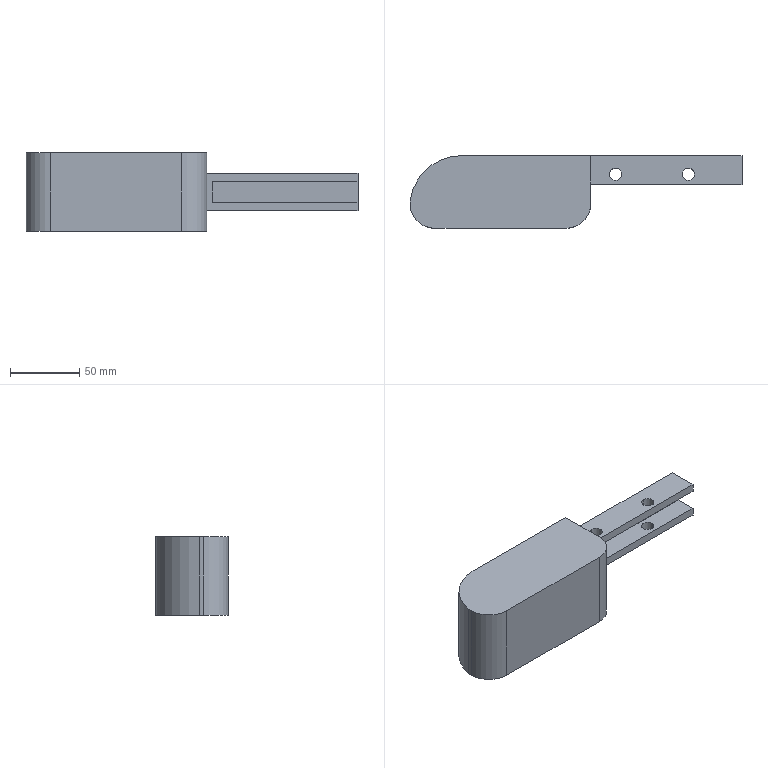Part | SolidWorks | features BaseBody 1, ICE 1 | 1 solid | 25 faces | box 239.768 x 52.5 x 57 mm | volume 402739 mm3 | plane 13 | cylinder 12 | commonest cylinder face diameters 9 x8 36 x3 75 x1
STEP:
#1=CARTESIAN_POINT('',(0.2322,-13.5,42.));
#2=VERTEX_POINT('',#1);
#3=CARTESIAN_POINT('',(18.232,-31.5,42.));
#4=VERTEX_POINT('',#3);
#5=CARTESIAN_POINT('',(18.232,-13.5,42.));
#6=DIRECTION('',(0.,0.,1.));
#7=DIRECTION('',(-1.,0.,0.));
#8=AXIS2_PLACEMENT_3D('',#5,#6,#7);
#9=CIRCLE('',#8,18.);
#10=EDGE_CURVE('',#2,#4,#9,.T.);
#11=ORIENTED_EDGE('',*,*,#10,.F.);
#12=CARTESIAN_POINT('',(0.2322,-13.5,-15.));
#13=VERTEX_POINT('',#12);
#14=CARTESIAN_POINT('',(0.2322,-13.5,42.));
#15=DIRECTION('',(0.,0.,-1.));
#16=VECTOR('',#15,1000.);
#17=LINE('',#14,#16);
#18=EDGE_CURVE('',#2,#13,#17,.T.);
#19=ORIENTED_EDGE('',*,*,#18,.T.);
#20=CARTESIAN_POINT('',(18.232,-31.5,-15.));
#21=VERTEX_POINT('',#20);
#22=CARTESIAN_POINT('',(18.232,-13.5,-15.));
#23=DIRECTION('',(0.,0.,-1.));
#24=DIRECTION('',(-1.,0.,0.));
#25=AXIS2_PLACEMENT_3D('',#22,#23,#24);
#26=CIRCLE('',#25,18.);
#27=EDGE_CURVE('',#21,#13,#26,.T.);
#28=ORIENTED_EDGE('',*,*,#27,.F.);
#29=CARTESIAN_POINT('',(18.232,-31.5,13.5));
#30=DIRECTION('',(0.,0.,-1.));
#31=VECTOR('',#30,1000.);
#32=LINE('',#29,#31);
#33=EDGE_CURVE('',#4,#21,#32,.T.);
#34=ORIENTED_EDGE('',*,*,#33,.F.);
#35=EDGE_LOOP('',(#11,#19,#28,#34));
#36=FACE_OUTER_BOUND('',#35,.T.);
#37=CARTESIAN_POINT('',(18.232,-13.5,42.));
#38=DIRECTION('',(0.,0.,-1.));
#39=DIRECTION('',(-1.,0.,0.));
#40=AXIS2_PLACEMENT_3D('',#37,#38,#39);
#41=CYLINDRICAL_SURFACE('',#40,18.);
#42=ADVANCED_FACE('',(#36),#41,.T.);
#43=CARTESIAN_POINT('',(144.21,7.5,6.));
#44=VERTEX_POINT('',#43);
#45=CARTESIAN_POINT('',(153.21,7.5,6.));
#46=VERTEX_POINT('',#45);
#47=CARTESIAN_POINT('',(148.71,7.5,6.));
#48=DIRECTION('',(0.,0.,1.));
#49=DIRECTION('',(-1.,0.,0.));
#50=AXIS2_PLACEMENT_3D('',#47,#48,#49);
#51=CIRCLE('',#50,4.5);
#52=EDGE_CURVE('',#44,#46,#51,.T.);
#53=ORIENTED_EDGE('',*,*,#52,.T.);
#54=CARTESIAN_POINT('',(153.21,7.5,0.));
#55=VERTEX_POINT('',#54);
#56=CARTESIAN_POINT('',(153.21,7.5,6.));
#57=DIRECTION('',(0.,0.,-1.));
#58=VECTOR('',#57,1000.);
#59=LINE('',#56,#58);
#60=EDGE_CURVE('',#46,#55,#59,.T.);
#61=ORIENTED_EDGE('',*,*,#60,.T.);
#62=CARTESIAN_POINT('',(144.21,7.5,0.));
#63=VERTEX_POINT('',#62);
#64=CARTESIAN_POINT('',(148.71,7.5,0.));
#65=DIRECTION('',(0.,0.,1.));
#66=DIRECTION('',(-1.,0.,0.));
#67=AXIS2_PLACEMENT_3D('',#64,#65,#66);
#68=CIRCLE('',#67,4.5);
#69=EDGE_CURVE('',#63,#55,#68,.T.);
#70=ORIENTED_EDGE('',*,*,#69,.F.);
#71=CARTESIAN_POINT('',(144.21,7.5,6.));
#72=DIRECTION('',(0.,0.,-1.));
#73=VECTOR('',#72,1000.);
#74=LINE('',#71,#73);
#75=EDGE_CURVE('',#44,#63,#74,.T.);
#76=ORIENTED_EDGE('',*,*,#75,.F.);
#77=EDGE_LOOP('',(#53,#61,#70,#76));
#78=FACE_OUTER_BOUND('',#77,.T.);
#79=CARTESIAN_POINT('',(148.71,7.5,6.));
#80=DIRECTION('',(0.,0.,-1.));
#81=DIRECTION('',(-1.,0.,0.));
#82=AXIS2_PLACEMENT_3D('',#79,#80,#81);
#83=CYLINDRICAL_SURFACE('',#82,4.5);
#84=ADVANCED_FACE('',(#78),#83,.F.);
#85=CARTESIAN_POINT('',(196.71,7.5,6.));
#86=VERTEX_POINT('',#85);
#87=CARTESIAN_POINT('',(205.71,7.5,6.));
#88=VERTEX_POINT('',#87);
#89=CARTESIAN_POINT('',(201.21,7.5,6.));
#90=DIRECTION('',(0.,0.,1.));
#91=DIRECTION('',(-1.,0.,0.));
#92=AXIS2_PLACEMENT_3D('',#89,#90,#91);
#93=CIRCLE('',#92,4.5);
#94=EDGE_CURVE('',#86,#88,#93,.T.);
#95=ORIENTED_EDGE('',*,*,#94,.T.);
#96=CARTESIAN_POINT('',(205.71,7.5,0.));
#97=VERTEX_POINT('',#96);
#98=CARTESIAN_POINT('',(205.71,7.5,6.));
#99=DIRECTION('',(0.,0.,-1.));
#100=VECTOR('',#99,1000.);
#101=LINE('',#98,#100);
#102=EDGE_CURVE('',#88,#97,#101,.T.);
#103=ORIENTED_EDGE('',*,*,#102,.T.);
#104=CARTESIAN_POINT('',(196.71,7.5,0.));
#105=VERTEX_POINT('',#104);
#106=CARTESIAN_POINT('',(201.21,7.5,0.));
#107=DIRECTION('',(0.,0.,1.));
#108=DIRECTION('',(-1.,0.,0.));
#109=AXIS2_PLACEMENT_3D('',#106,#107,#108);
#110=CIRCLE('',#109,4.5);
#111=EDGE_CURVE('',#105,#97,#110,.T.);
#112=ORIENTED_EDGE('',*,*,#111,.F.);
#113=CARTESIAN_POINT('',(196.71,7.5,6.));
#114=DIRECTION('',(0.,0.,-1.));
#115=VECTOR('',#114,1000.);
#116=LINE('',#113,#115);
#117=EDGE_CURVE('',#86,#105,#116,.T.);
#118=ORIENTED_EDGE('',*,*,#117,.F.);
#119=EDGE_LOOP('',(#95,#103,#112,#118));
#120=FACE_OUTER_BOUND('',#119,.T.);
#121=CARTESIAN_POINT('',(201.21,7.5,6.));
#122=DIRECTION('',(0.,0.,-1.));
#123=DIRECTION('',(-1.,0.,0.));
#124=AXIS2_PLACEMENT_3D('',#121,#122,#123);
#125=CYLINDRICAL_SURFACE('',#124,4.5);
#126=ADVANCED_FACE('',(#120),#125,.F.);
#127=CARTESIAN_POINT('',(148.71,12.,27.));
#128=VERTEX_POINT('',#127);
#129=CARTESIAN_POINT('',(148.71,3.,27.));
#130=VERTEX_POINT('',#129);
#131=CARTESIAN_POINT('',(148.71,7.5,27.));
#132=DIRECTION('',(0.,0.,1.));
#133=DIRECTION('',(0.,1.,0.));
#134=AXIS2_PLACEMENT_3D('',#131,#132,#133);
#135=CIRCLE('',#134,4.5);
#136=EDGE_CURVE('',#128,#130,#135,.T.);
#137=ORIENTED_EDGE('',*,*,#136,.T.);
#138=CARTESIAN_POINT('',(148.71,3.,21.));
#139=VERTEX_POINT('',#138);
#140=CARTESIAN_POINT('',(148.71,3.,27.));
#141=DIRECTION('',(0.,0.,-1.));
#142=VECTOR('',#141,1000.);
#143=LINE('',#140,#142);
#144=EDGE_CURVE('',#130,#139,#143,.T.);
#145=ORIENTED_EDGE('',*,*,#144,.T.);
#146=CARTESIAN_POINT('',(148.71,12.,21.));
#147=VERTEX_POINT('',#146);
#148=CARTESIAN_POINT('',(148.71,7.5,21.));
#149=DIRECTION('',(0.,0.,-1.));
#150=DIRECTION('',(0.,1.,0.));
#151=AXIS2_PLACEMENT_3D('',#148,#149,#150);
#152=CIRCLE('',#151,4.5);
#153=EDGE_CURVE('',#139,#147,#152,.T.);
#154=ORIENTED_EDGE('',*,*,#153,.T.);
#155=CARTESIAN_POINT('',(148.71,12.,27.));
#156=DIRECTION('',(0.,0.,-1.));
#157=VECTOR('',#156,1000.);
#158=LINE('',#155,#157);
#159=EDGE_CURVE('',#128,#147,#158,.T.);
#160=ORIENTED_EDGE('',*,*,#159,.F.);
#161=EDGE_LOOP('',(#137,#145,#154,#160));
#162=FACE_OUTER_BOUND('',#161,.T.);
#163=CARTESIAN_POINT('',(148.71,7.5,27.));
#164=DIRECTION('',(0.,0.,-1.));
#165=DIRECTION('',(0.,1.,0.));
#166=AXIS2_PLACEMENT_3D('',#163,#164,#165);
#167=CYLINDRICAL_SURFACE('',#166,4.5);
#168=ADVANCED_FACE('',(#162),#167,.F.);
#169=CARTESIAN_POINT('',(201.21,12.,27.));
#170=VERTEX_POINT('',#169);
#171=CARTESIAN_POINT('',(201.21,3.,27.));
#172=VERTEX_POINT('',#171);
#173=CARTESIAN_POINT('',(201.21,7.5,27.));
#174=DIRECTION('',(0.,0.,1.));
#175=DIRECTION('',(0.,1.,0.));
#176=AXIS2_PLACEMENT_3D('',#173,#174,#175);
#177=CIRCLE('',#176,4.5);
#178=EDGE_CURVE('',#170,#172,#177,.T.);
#179=ORIENTED_EDGE('',*,*,#178,.T.);
#180=CARTESIAN_POINT('',(201.21,3.,21.));
#181=VERTEX_POINT('',#180);
#182=CARTESIAN_POINT('',(201.21,3.,27.));
#183=DIRECTION('',(0.,0.,-1.));
#184=VECTOR('',#183,1000.);
#185=LINE('',#182,#184);
#186=EDGE_CURVE('',#172,#181,#185,.T.);
#187=ORIENTED_EDGE('',*,*,#186,.T.);
#188=CARTESIAN_POINT('',(201.21,12.,21.));
#189=VERTEX_POINT('',#188);
#190=CARTESIAN_POINT('',(201.21,7.5,21.));
#191=DIRECTION('',(0.,0.,-1.));
#192=DIRECTION('',(0.,1.,0.));
#193=AXIS2_PLACEMENT_3D('',#190,#191,#192);
#194=CIRCLE('',#193,4.5);
#195=EDGE_CURVE('',#181,#189,#194,.T.);
#196=ORIENTED_EDGE('',*,*,#195,.T.);
#197=CARTESIAN_POINT('',(201.21,12.,27.));
#198=DIRECTION('',(0.,0.,-1.));
#199=VECTOR('',#198,1000.);
#200=LINE('',#197,#199);
#201=EDGE_CURVE('',#170,#189,#200,.T.);
#202=ORIENTED_EDGE('',*,*,#201,.F.);
#203=EDGE_LOOP('',(#179,#187,#196,#202));
#204=FACE_OUTER_BOUND('',#203,.T.);
#205=CARTESIAN_POINT('',(201.21,7.5,27.));
#206=DIRECTION('',(0.,0.,-1.));
#207=DIRECTION('',(0.,1.,0.));
#208=AXIS2_PLACEMENT_3D('',#205,#206,#207);
#209=CYLINDRICAL_SURFACE('',#208,4.5);
#210=ADVANCED_FACE('',(#204),#209,.F.);
#211=ORIENTED_EDGE('',*,*,#18,.F.);
#212=CARTESIAN_POINT('',(0.4464,-10.731,42.));
#213=VERTEX_POINT('',#212);
#214=CARTESIAN_POINT('',(18.232,-13.5,42.));
#215=DIRECTION('',(0.,0.,1.));
#216=DIRECTION('',(-1.,0.,0.));
#217=AXIS2_PLACEMENT_3D('',#214,#215,#216);
#218=CIRCLE('',#217,18.);
#219=EDGE_CURVE('',#213,#2,#218,.T.);
#220=ORIENTED_EDGE('',*,*,#219,.F.);
#221=CARTESIAN_POINT('',(0.4464,-10.731,-15.));
#222=VERTEX_POINT('',#221);
#223=CARTESIAN_POINT('',(0.4464,-10.731,13.5));
#224=DIRECTION('',(0.,0.,1.));
#225=VECTOR('',#224,1000.);
#226=LINE('',#223,#225);
#227=EDGE_CURVE('',#222,#213,#226,.T.);
#228=ORIENTED_EDGE('',*,*,#227,.F.);
#229=CARTESIAN_POINT('',(18.232,-13.5,-15.));
#230=DIRECTION('',(0.,0.,-1.));
#231=DIRECTION('',(-1.,0.,0.));
#232=AXIS2_PLACEMENT_3D('',#229,#230,#231);
#233=CIRCLE('',#232,18.);
#234=EDGE_CURVE('',#13,#222,#233,.T.);
#235=ORIENTED_EDGE('',*,*,#234,.F.);
#236=EDGE_LOOP('',(#211,#220,#228,#235));
#237=FACE_OUTER_BOUND('',#236,.T.);
#238=CARTESIAN_POINT('',(18.232,-13.5,42.));
#239=DIRECTION('',(0.,0.,-1.));
#240=DIRECTION('',(-1.,0.,0.));
#241=AXIS2_PLACEMENT_3D('',#238,#239,#240);
#242=CYLINDRICAL_SURFACE('',#241,18.);
#243=ADVANCED_FACE('',(#237),#242,.T.);
#244=CARTESIAN_POINT('',(130.767,21.,42.));
#245=VERTEX_POINT('',#244);
#246=CARTESIAN_POINT('',(130.767,-13.5,42.));
#247=VERTEX_POINT('',#246);
#248=CARTESIAN_POINT('',(130.767,-5.25,42.));
#249=DIRECTION('',(0.,-1.,0.));
#250=VECTOR('',#249,1000.);
#251=LINE('',#248,#250);
#252=EDGE_CURVE('',#245,#247,#251,.T.);
#253=ORIENTED_EDGE('',*,*,#252,.F.);
#254=CARTESIAN_POINT('',(37.5,21.,42.));
#255=VERTEX_POINT('',#254);
#256=CARTESIAN_POINT('',(65.108,21.,42.));
#257=DIRECTION('',(1.,0.,0.));
#258=VECTOR('',#257,1000.);
#259=LINE('',#256,#258);
#260=EDGE_CURVE('',#255,#245,#259,.T.);
#261=ORIENTED_EDGE('',*,*,#260,.F.);
#262=CARTESIAN_POINT('',(37.5,-16.5,42.));
#263=DIRECTION('',(0.,0.,-1.));
#264=DIRECTION('',(-1.,0.,0.));
#265=AXIS2_PLACEMENT_3D('',#262,#263,#264);
#266=CIRCLE('',#265,37.5);
#267=EDGE_CURVE('',#213,#255,#266,.T.);
#268=ORIENTED_EDGE('',*,*,#267,.F.);
#269=ORIENTED_EDGE('',*,*,#219,.T.);
#270=ORIENTED_EDGE('',*,*,#10,.T.);
#271=CARTESIAN_POINT('',(112.767,-31.5,42.));
#272=VERTEX_POINT('',#271);
#273=CARTESIAN_POINT('',(65.108,-31.5,42.));
#274=DIRECTION('',(-1.,0.,0.));
#275=VECTOR('',#274,1000.);
#276=LINE('',#273,#275);
#277=EDGE_CURVE('',#272,#4,#276,.T.);
#278=ORIENTED_EDGE('',*,*,#277,.F.);
#279=CARTESIAN_POINT('',(112.767,-13.5,42.));
#280=DIRECTION('',(0.,0.,-1.));
#281=DIRECTION('',(-1.,0.,0.));
#282=AXIS2_PLACEMENT_3D('',#279,#280,#281);
#283=CIRCLE('',#282,18.);
#284=EDGE_CURVE('',#247,#272,#283,.T.);
#285=ORIENTED_EDGE('',*,*,#284,.F.);
#286=EDGE_LOOP('',(#253,#261,#268,#269,#270,#278,#285));
#287=FACE_OUTER_BOUND('',#286,.T.);
#288=CARTESIAN_POINT('',(130.767,-31.5,42.));
#289=DIRECTION('',(0.,0.,-1.));
#290=DIRECTION('',(-1.,0.,0.));
#291=AXIS2_PLACEMENT_3D('',#288,#289,#290);
#292=PLANE('',#291);
#293=ADVANCED_FACE('',(#287),#292,.F.);
#294=CARTESIAN_POINT('',(112.767,-31.5,-15.));
#295=VERTEX_POINT('',#294);
#296=CARTESIAN_POINT('',(65.108,-31.5,-15.));
#297=DIRECTION('',(1.,0.,0.));
#298=VECTOR('',#297,1000.);
#299=LINE('',#296,#298);
#300=EDGE_CURVE('',#21,#295,#299,.T.);
#301=ORIENTED_EDGE('',*,*,#300,.F.);
#302=ORIENTED_EDGE('',*,*,#27,.T.);
#303=ORIENTED_EDGE('',*,*,#234,.T.);
#304=CARTESIAN_POINT('',(37.5,21.,-15.));
#305=VERTEX_POINT('',#304);
#306=CARTESIAN_POINT('',(37.5,-16.5,-15.));
#307=DIRECTION('',(0.,0.,1.));
#308=DIRECTION('',(-1.,0.,0.));
#309=AXIS2_PLACEMENT_3D('',#306,#307,#308);
#310=CIRCLE('',#309,37.5);
#311=EDGE_CURVE('',#305,#222,#310,.T.);
#312=ORIENTED_EDGE('',*,*,#311,.F.);
#313=CARTESIAN_POINT('',(130.767,21.,-15.));
#314=VERTEX_POINT('',#313);
#315=CARTESIAN_POINT('',(65.108,21.,-15.));
#316=DIRECTION('',(-1.,0.,0.));
#317=VECTOR('',#316,1000.);
#318=LINE('',#315,#317);
#319=EDGE_CURVE('',#314,#305,#318,.T.);
#320=ORIENTED_EDGE('',*,*,#319,.F.);
#321=CARTESIAN_POINT('',(130.767,-13.5,-15.));
#322=VERTEX_POINT('',#321);
#323=CARTESIAN_POINT('',(130.767,-5.25,-15.));
#324=DIRECTION('',(0.,1.,0.));
#325=VECTOR('',#324,1000.);
#326=LINE('',#323,#325);
#327=EDGE_CURVE('',#322,#314,#326,.T.);
#328=ORIENTED_EDGE('',*,*,#327,.F.);
#329=CARTESIAN_POINT('',(112.767,-13.5,-15.));
#330=DIRECTION('',(0.,0.,1.));
#331=DIRECTION('',(-1.,0.,0.));
#332=AXIS2_PLACEMENT_3D('',#329,#330,#331);
#333=CIRCLE('',#332,18.);
#334=EDGE_CURVE('',#295,#322,#333,.T.);
#335=ORIENTED_EDGE('',*,*,#334,.F.);
#336=EDGE_LOOP('',(#301,#302,#303,#312,#320,#328,#335));
#337=FACE_OUTER_BOUND('',#336,.T.);
#338=CARTESIAN_POINT('',(-0.5511,-31.5,-15.));
#339=DIRECTION('',(0.,0.,1.));
#340=DIRECTION('',(1.,0.,0.));
#341=AXIS2_PLACEMENT_3D('',#338,#339,#340);
#342=PLANE('',#341);
#343=ADVANCED_FACE('',(#337),#342,.F.);
#344=ORIENTED_EDGE('',*,*,#33,.T.);
#345=ORIENTED_EDGE('',*,*,#300,.T.);
#346=CARTESIAN_POINT('',(112.767,-31.5,13.5));
#347=DIRECTION('',(0.,0.,1.));
#348=VECTOR('',#347,1000.);
#349=LINE('',#346,#348);
#350=EDGE_CURVE('',#295,#272,#349,.T.);
#351=ORIENTED_EDGE('',*,*,#350,.T.);
#352=ORIENTED_EDGE('',*,*,#277,.T.);
#353=EDGE_LOOP('',(#344,#345,#351,#352));
#354=FACE_OUTER_BOUND('',#353,.T.);
#355=CARTESIAN_POINT('',(18.232,-31.5,-15.));
#356=DIRECTION('',(0.,1.,0.));
#357=DIRECTION('',(0.,0.,1.));
#358=AXIS2_PLACEMENT_3D('',#355,#356,#357);
#359=PLANE('',#358);
#360=ADVANCED_FACE('',(#354),#359,.F.);
#361=CARTESIAN_POINT('',(130.767,-13.5,13.5));
#362=DIRECTION('',(0.,0.,-1.));
#363=VECTOR('',#362,1000.);
#364=LINE('',#361,#363);
#365=EDGE_CURVE('',#247,#322,#364,.T.);
#366=ORIENTED_EDGE('',*,*,#365,.F.);
#367=ORIENTED_EDGE('',*,*,#284,.T.);
#368=ORIENTED_EDGE('',*,*,#350,.F.);
#369=ORIENTED_EDGE('',*,*,#334,.T.);
#370=EDGE_LOOP('',(#366,#367,#368,#369));
#371=FACE_OUTER_BOUND('',#370,.T.);
#372=CARTESIAN_POINT('',(112.767,-13.5,42.));
#373=DIRECTION('',(0.,0.,-1.));
#374=DIRECTION('',(-1.,0.,0.));
#375=AXIS2_PLACEMENT_3D('',#372,#373,#374);
#376=CYLINDRICAL_SURFACE('',#375,18.);
#377=ADVANCED_FACE('',(#371),#376,.T.);
#378=ORIENTED_EDGE('',*,*,#327,.T.);
#379=CARTESIAN_POINT('',(130.767,21.,0.000000015));
#380=VERTEX_POINT('',#379);
#381=CARTESIAN_POINT('',(130.767,21.,13.5));
#382=DIRECTION('',(0.,0.,-1.));
#383=VECTOR('',#382,1000.);
#384=LINE('',#381,#383);
#385=EDGE_CURVE('',#380,#314,#384,.T.);
#386=ORIENTED_EDGE('',*,*,#385,.F.);
#387=CARTESIAN_POINT('',(130.767,0.000000004,0.00000001));
#388=VERTEX_POINT('',#387);
#389=CARTESIAN_POINT('',(130.767,3.75,0.000000015));
#390=DIRECTION('',(0.,1.,0.));
#391=VECTOR('',#390,1000.);
#392=LINE('',#389,#391);
#393=EDGE_CURVE('',#388,#380,#392,.T.);
#394=ORIENTED_EDGE('',*,*,#393,.F.);
#395=CARTESIAN_POINT('',(130.767,0.000000004,27.));
#396=VERTEX_POINT('',#395);
#397=CARTESIAN_POINT('',(130.767,0.000000006,13.5));
#398=DIRECTION('',(0.,0.,-1.));
#399=VECTOR('',#398,1000.);
#400=LINE('',#397,#399);
#401=EDGE_CURVE('',#396,#388,#400,.T.);
#402=ORIENTED_EDGE('',*,*,#401,.F.);
#403=CARTESIAN_POINT('',(130.767,21.,27.));
#404=VERTEX_POINT('',#403);
#405=CARTESIAN_POINT('',(130.767,3.75,27.));
#406=DIRECTION('',(0.,-1.,0.));
#407=VECTOR('',#406,1000.);
#408=LINE('',#405,#407);
#409=EDGE_CURVE('',#404,#396,#408,.T.);
#410=ORIENTED_EDGE('',*,*,#409,.F.);
#411=CARTESIAN_POINT('',(130.767,21.,13.5));
#412=DIRECTION('',(0.,0.,-1.));
#413=VECTOR('',#412,1000.);
#414=LINE('',#411,#413);
#415=EDGE_CURVE('',#245,#404,#414,.T.);
#416=ORIENTED_EDGE('',*,*,#415,.F.);
#417=ORIENTED_EDGE('',*,*,#252,.T.);
#418=ORIENTED_EDGE('',*,*,#365,.T.);
#419=EDGE_LOOP('',(#378,#386,#394,#402,#410,#416,#417,#418));
#420=FACE_OUTER_BOUND('',#419,.T.);
#421=CARTESIAN_POINT('',(130.767,-13.5,-15.));
#422=DIRECTION('',(-1.,0.,0.));
#423=DIRECTION('',(0.,0.,1.));
#424=AXIS2_PLACEMENT_3D('',#421,#422,#423);
#425=PLANE('',#424);
#426=ADVANCED_FACE('',(#420),#425,.F.);
#427=ORIENTED_EDGE('',*,*,#260,.T.);
#428=ORIENTED_EDGE('',*,*,#415,.T.);
#429=CARTESIAN_POINT('',(240.,21.,27.));
#430=VERTEX_POINT('',#429);
#431=CARTESIAN_POINT('',(138.75,21.,27.));
#432=DIRECTION('',(-1.,0.,0.));
#433=VECTOR('',#432,1000.);
#434=LINE('',#431,#433);
#435=EDGE_CURVE('',#430,#404,#434,.T.);
#436=ORIENTED_EDGE('',*,*,#435,.F.);
#437=CARTESIAN_POINT('',(240.,21.,0.00000001));
#438=VERTEX_POINT('',#437);
#439=CARTESIAN_POINT('',(240.,21.,13.5));
#440=DIRECTION('',(0.,0.,1.));
#441=VECTOR('',#440,1000.);
#442=LINE('',#439,#441);
#443=EDGE_CURVE('',#438,#430,#442,.T.);
#444=ORIENTED_EDGE('',*,*,#443,.F.);
#445=CARTESIAN_POINT('',(138.75,21.,0.000000015));
#446=DIRECTION('',(1.,0.,0.));
#447=VECTOR('',#446,1000.);
#448=LINE('',#445,#447);
#449=EDGE_CURVE('',#380,#438,#448,.T.);
#450=ORIENTED_EDGE('',*,*,#449,.F.);
#451=ORIENTED_EDGE('',*,*,#385,.T.);
#452=ORIENTED_EDGE('',*,*,#319,.T.);
#453=CARTESIAN_POINT('',(37.5,21.,13.5));
#454=DIRECTION('',(0.,0.,-1.));
#455=VECTOR('',#454,1000.);
#456=LINE('',#453,#455);
#457=EDGE_CURVE('',#255,#305,#456,.T.);
#458=ORIENTED_EDGE('',*,*,#457,.F.);
#459=EDGE_LOOP('',(#427,#428,#436,#444,#450,#451,#452,#458));
#460=FACE_OUTER_BOUND('',#459,.T.);
#461=CARTESIAN_POINT('',(37.5,21.,42.));
#462=DIRECTION('',(0.,-1.,0.));
#463=DIRECTION('',(0.,0.,-1.));
#464=AXIS2_PLACEMENT_3D('',#461,#462,#463);
#465=PLANE('',#464);
#466=ADVANCED_FACE('',(#460),#465,.F.);
#467=ORIENTED_EDGE('',*,*,#457,.T.);
#468=ORIENTED_EDGE('',*,*,#311,.T.);
#469=ORIENTED_EDGE('',*,*,#227,.T.);
#470=ORIENTED_EDGE('',*,*,#267,.T.);
#471=EDGE_LOOP('',(#467,#468,#469,#470));
#472=FACE_OUTER_BOUND('',#471,.T.);
#473=CARTESIAN_POINT('',(37.5,-16.5,42.));
#474=DIRECTION('',(0.,0.,-1.));
#475=DIRECTION('',(-1.,0.,0.));
#476=AXIS2_PLACEMENT_3D('',#473,#474,#475);
#477=CYLINDRICAL_SURFACE('',#476,37.5);
#478=ADVANCED_FACE('',(#472),#477,.T.);
#479=ORIENTED_EDGE('',*,*,#69,.T.);
#480=CARTESIAN_POINT('',(148.71,7.5,0.));
#481=DIRECTION('',(0.,0.,1.));
#482=DIRECTION('',(-1.,0.,0.));
#483=AXIS2_PLACEMENT_3D('',#480,#481,#482);
#484=CIRCLE('',#483,4.5);
#485=EDGE_CURVE('',#55,#63,#484,.T.);
#486=ORIENTED_EDGE('',*,*,#485,.T.);
#487=EDGE_LOOP('',(#479,#486));
#488=FACE_BOUND('',#487,.T.);
#489=ORIENTED_EDGE('',*,*,#111,.T.);
#490=CARTESIAN_POINT('',(201.21,7.5,0.));
#491=DIRECTION('',(0.,0.,1.));
#492=DIRECTION('',(-1.,0.,0.));
#493=AXIS2_PLACEMENT_3D('',#490,#491,#492);
#494=CIRCLE('',#493,4.5);
#495=EDGE_CURVE('',#97,#105,#494,.T.);
#496=ORIENTED_EDGE('',*,*,#495,.T.);
#497=EDGE_LOOP('',(#489,#496));
#498=FACE_BOUND('',#497,.T.);
#499=ORIENTED_EDGE('',*,*,#393,.T.);
#500=ORIENTED_EDGE('',*,*,#449,.T.);
#501=CARTESIAN_POINT('',(240.,0.,0.));
#502=VERTEX_POINT('',#501);
#503=CARTESIAN_POINT('',(240.,10.5,0.));
#504=DIRECTION('',(0.,-1.,0.));
#505=VECTOR('',#504,1000.);
#506=LINE('',#503,#505);
#507=EDGE_CURVE('',#438,#502,#506,.T.);
#508=ORIENTED_EDGE('',*,*,#507,.T.);
#509=CARTESIAN_POINT('',(185.384,0.,0.));
#510=DIRECTION('',(-1.,0.,0.));
#511=VECTOR('',#510,1000.);
#512=LINE('',#509,#511);
#513=EDGE_CURVE('',#502,#388,#512,.T.);
#514=ORIENTED_EDGE('',*,*,#513,.T.);
#515=EDGE_LOOP('',(#499,#500,#508,#514));
#516=FACE_OUTER_BOUND('',#515,.T.);
#517=CARTESIAN_POINT('',(240.,0.,0.));
#518=DIRECTION('',(0.,0.,-1.));
#519=DIRECTION('',(-1.,0.,0.));
#520=AXIS2_PLACEMENT_3D('',#517,#518,#519);
#521=PLANE('',#520);
#522=ADVANCED_FACE('',(#488,#498,#516),#521,.T.);
#523=ORIENTED_EDGE('',*,*,#401,.T.);
#524=ORIENTED_EDGE('',*,*,#513,.F.);
#525=CARTESIAN_POINT('',(240.,0.,6.));
#526=VERTEX_POINT('',#525);
#527=CARTESIAN_POINT('',(240.,0.,13.5));
#528=DIRECTION('',(0.,0.,-1.));
#529=VECTOR('',#528,1000.);
#530=LINE('',#527,#529);
#531=EDGE_CURVE('',#526,#502,#530,.T.);
#532=ORIENTED_EDGE('',*,*,#531,.F.);
#533=CARTESIAN_POINT('',(135.,0.,6.));
#534=VERTEX_POINT('',#533);
#535=CARTESIAN_POINT('',(185.384,0.,6.));
#536=DIRECTION('',(1.,0.,0.));
#537=VECTOR('',#536,1000.);
#538=LINE('',#535,#537);
#539=EDGE_CURVE('',#534,#526,#538,.T.);
#540=ORIENTED_EDGE('',*,*,#539,.F.);
#541=CARTESIAN_POINT('',(135.,0.,21.));
#542=VERTEX_POINT('',#541);
#543=CARTESIAN_POINT('',(135.,0.,13.5));
#544=DIRECTION('',(0.,0.,-1.));
#545=VECTOR('',#544,1000.);
#546=LINE('',#543,#545);
#547=EDGE_CURVE('',#542,#534,#546,.T.);
#548=ORIENTED_EDGE('',*,*,#547,.F.);
#549=CARTESIAN_POINT('',(240.,0.,21.));
#550=VERTEX_POINT('',#549);
#551=CARTESIAN_POINT('',(185.384,0.,21.));
#552=DIRECTION('',(-1.,0.,0.));
#553=VECTOR('',#552,1000.);
#554=LINE('',#551,#553);
#555=EDGE_CURVE('',#550,#542,#554,.T.);
#556=ORIENTED_EDGE('',*,*,#555,.F.);
#557=CARTESIAN_POINT('',(240.,0.,27.));
#558=VERTEX_POINT('',#557);
#559=CARTESIAN_POINT('',(240.,0.,13.5));
#560=DIRECTION('',(0.,0.,-1.));
#561=VECTOR('',#560,1000.);
#562=LINE('',#559,#561);
#563=EDGE_CURVE('',#558,#550,#562,.T.);
#564=ORIENTED_EDGE('',*,*,#563,.F.);
#565=CARTESIAN_POINT('',(185.384,0.,27.));
#566=DIRECTION('',(1.,0.,0.));
#567=VECTOR('',#566,1000.);
#568=LINE('',#565,#567);
#569=EDGE_CURVE('',#396,#558,#568,.T.);
#570=ORIENTED_EDGE('',*,*,#569,.F.);
#571=EDGE_LOOP('',(#523,#524,#532,#540,#548,#556,#564,#570));
#572=FACE_OUTER_BOUND('',#571,.T.);
#573=CARTESIAN_POINT('',(130.767,0.,0.));
#574=DIRECTION('',(0.,1.,0.));
#575=DIRECTION('',(0.,0.,1.));
#576=AXIS2_PLACEMENT_3D('',#573,#574,#575);
#577=PLANE('',#576);
#578=ADVANCED_FACE('',(#572),#577,.F.);
#579=ORIENTED_EDGE('',*,*,#136,.F.);
#580=CARTESIAN_POINT('',(148.71,7.5,27.));
#581=DIRECTION('',(0.,0.,1.));
#582=DIRECTION('',(0.,1.,0.));
#583=AXIS2_PLACEMENT_3D('',#580,#581,#582);
#584=CIRCLE('',#583,4.5);
#585=EDGE_CURVE('',#130,#128,#584,.T.);
#586=ORIENTED_EDGE('',*,*,#585,.F.);
#587=EDGE_LOOP('',(#579,#586));
#588=FACE_BOUND('',#587,.T.);
#589=ORIENTED_EDGE('',*,*,#178,.F.);
#590=CARTESIAN_POINT('',(201.21,7.5,27.));
#591=DIRECTION('',(0.,0.,1.));
#592=DIRECTION('',(0.,1.,0.));
#593=AXIS2_PLACEMENT_3D('',#590,#591,#592);
#594=CIRCLE('',#593,4.5);
#595=EDGE_CURVE('',#172,#170,#594,.T.);
#596=ORIENTED_EDGE('',*,*,#595,.F.);
#597=EDGE_LOOP('',(#589,#596));
#598=FACE_BOUND('',#597,.T.);
#599=ORIENTED_EDGE('',*,*,#569,.T.);
#600=CARTESIAN_POINT('',(240.,10.5,27.));
#601=DIRECTION('',(0.,-1.,0.));
#602=VECTOR('',#601,1000.);
#603=LINE('',#600,#602);
#604=EDGE_CURVE('',#430,#558,#603,.T.);
#605=ORIENTED_EDGE('',*,*,#604,.F.);
#606=ORIENTED_EDGE('',*,*,#435,.T.);
#607=ORIENTED_EDGE('',*,*,#409,.T.);
#608=EDGE_LOOP('',(#599,#605,#606,#607));
#609=FACE_OUTER_BOUND('',#608,.T.);
#610=CARTESIAN_POINT('',(240.,0.,27.));
#611=DIRECTION('',(0.,0.,-1.));
#612=DIRECTION('',(-1.,0.,0.));
#613=AXIS2_PLACEMENT_3D('',#610,#611,#612);
#614=PLANE('',#613);
#615=ADVANCED_FACE('',(#588,#598,#609),#614,.F.);
#616=ORIENTED_EDGE('',*,*,#604,.T.);
#617=ORIENTED_EDGE('',*,*,#563,.T.);
#618=CARTESIAN_POINT('',(240.,15.,21.));
#619=VERTEX_POINT('',#618);
#620=CARTESIAN_POINT('',(240.,10.5,21.));
#621=DIRECTION('',(0.,-1.,0.));
#622=VECTOR('',#621,1000.);
#623=LINE('',#620,#622);
#624=EDGE_CURVE('',#619,#550,#623,.T.);
#625=ORIENTED_EDGE('',*,*,#624,.F.);
#626=CARTESIAN_POINT('',(240.,15.,6.));
#627=VERTEX_POINT('',#626);
#628=CARTESIAN_POINT('',(240.,15.,13.5));
#629=DIRECTION('',(0.,0.,1.));
#630=VECTOR('',#629,1000.);
#631=LINE('',#628,#630);
#632=EDGE_CURVE('',#627,#619,#631,.T.);
#633=ORIENTED_EDGE('',*,*,#632,.F.);
#634=CARTESIAN_POINT('',(240.,10.5,6.));
#635=DIRECTION('',(0.,1.,0.));
#636=VECTOR('',#635,1000.);
#637=LINE('',#634,#636);
#638=EDGE_CURVE('',#526,#627,#637,.T.);
#639=ORIENTED_EDGE('',*,*,#638,.F.);
#640=ORIENTED_EDGE('',*,*,#531,.T.);
#641=ORIENTED_EDGE('',*,*,#507,.F.);
#642=ORIENTED_EDGE('',*,*,#443,.T.);
#643=EDGE_LOOP('',(#616,#617,#625,#633,#639,#640,#641,#642));
#644=FACE_OUTER_BOUND('',#643,.T.);
#645=CARTESIAN_POINT('',(240.,0.,0.));
#646=DIRECTION('',(-1.,0.,0.));
#647=DIRECTION('',(0.,0.,1.));
#648=AXIS2_PLACEMENT_3D('',#645,#646,#647);
#649=PLANE('',#648);
#650=ADVANCED_FACE('',(#644),#649,.F.);
#651=ORIENTED_EDGE('',*,*,#60,.F.);
#652=CARTESIAN_POINT('',(148.71,7.5,6.));
#653=DIRECTION('',(0.,0.,1.));
#654=DIRECTION('',(-1.,0.,0.));
#655=AXIS2_PLACEMENT_3D('',#652,#653,#654);
#656=CIRCLE('',#655,4.5);
#657=EDGE_CURVE('',#46,#44,#656,.T.);
#658=ORIENTED_EDGE('',*,*,#657,.T.);
#659=ORIENTED_EDGE('',*,*,#75,.T.);
#660=ORIENTED_EDGE('',*,*,#485,.F.);
#661=EDGE_LOOP('',(#651,#658,#659,#660));
#662=FACE_OUTER_BOUND('',#661,.T.);
#663=CARTESIAN_POINT('',(148.71,7.5,6.));
#664=DIRECTION('',(0.,0.,-1.));
#665=DIRECTION('',(-1.,0.,0.));
#666=AXIS2_PLACEMENT_3D('',#663,#664,#665);
#667=CYLINDRICAL_SURFACE('',#666,4.5);
#668=ADVANCED_FACE('',(#662),#667,.F.);
#669=ORIENTED_EDGE('',*,*,#102,.F.);
#670=CARTESIAN_POINT('',(201.21,7.5,6.));
#671=DIRECTION('',(0.,0.,1.));
#672=DIRECTION('',(-1.,0.,0.));
#673=AXIS2_PLACEMENT_3D('',#670,#671,#672);
#674=CIRCLE('',#673,4.5);
#675=EDGE_CURVE('',#88,#86,#674,.T.);
#676=ORIENTED_EDGE('',*,*,#675,.T.);
#677=ORIENTED_EDGE('',*,*,#117,.T.);
#678=ORIENTED_EDGE('',*,*,#495,.F.);
#679=EDGE_LOOP('',(#669,#676,#677,#678));
#680=FACE_OUTER_BOUND('',#679,.T.);
#681=CARTESIAN_POINT('',(201.21,7.5,6.));
#682=DIRECTION('',(0.,0.,-1.));
#683=DIRECTION('',(-1.,0.,0.));
#684=AXIS2_PLACEMENT_3D('',#681,#682,#683);
#685=CYLINDRICAL_SURFACE('',#684,4.5);
#686=ADVANCED_FACE('',(#680),#685,.F.);
#687=ORIENTED_EDGE('',*,*,#52,.F.);
#688=ORIENTED_EDGE('',*,*,#657,.F.);
#689=EDGE_LOOP('',(#687,#688));
#690=FACE_BOUND('',#689,.T.);
#691=ORIENTED_EDGE('',*,*,#94,.F.);
#692=ORIENTED_EDGE('',*,*,#675,.F.);
#693=EDGE_LOOP('',(#691,#692));
#694=FACE_BOUND('',#693,.T.);
#695=CARTESIAN_POINT('',(135.,15.,6.));
#696=VERTEX_POINT('',#695);
#697=CARTESIAN_POINT('',(135.,7.5,6.));
#698=DIRECTION('',(0.,1.,0.));
#699=VECTOR('',#698,1000.);
#700=LINE('',#697,#699);
#701=EDGE_CURVE('',#534,#696,#700,.T.);
#702=ORIENTED_EDGE('',*,*,#701,.F.);
#703=ORIENTED_EDGE('',*,*,#539,.T.);
#704=ORIENTED_EDGE('',*,*,#638,.T.);
#705=CARTESIAN_POINT('',(187.5,15.,6.));
#706=DIRECTION('',(1.,0.,0.));
#707=VECTOR('',#706,1000.);
#708=LINE('',#705,#707);
#709=EDGE_CURVE('',#696,#627,#708,.T.);
#710=ORIENTED_EDGE('',*,*,#709,.F.);
#711=EDGE_LOOP('',(#702,#703,#704,#710));
#712=FACE_OUTER_BOUND('',#711,.T.);
#713=CARTESIAN_POINT('',(240.,0.,6.));
#714=DIRECTION('',(0.,0.,-1.));
#715=DIRECTION('',(-1.,0.,0.));
#716=AXIS2_PLACEMENT_3D('',#713,#714,#715);
#717=PLANE('',#716);
#718=ADVANCED_FACE('',(#690,#694,#712),#717,.F.);
#719=ORIENTED_EDGE('',*,*,#701,.T.);
#720=CARTESIAN_POINT('',(135.,15.,21.));
#721=VERTEX_POINT('',#720);
#722=CARTESIAN_POINT('',(135.,15.,13.5));
#723=DIRECTION('',(0.,0.,-1.));
#724=VECTOR('',#723,1000.);
#725=LINE('',#722,#724);
#726=EDGE_CURVE('',#721,#696,#725,.T.);
#727=ORIENTED_EDGE('',*,*,#726,.F.);
#728=CARTESIAN_POINT('',(135.,7.5,21.));
#729=DIRECTION('',(0.,1.,0.));
#730=VECTOR('',#729,1000.);
#731=LINE('',#728,#730);
#732=EDGE_CURVE('',#542,#721,#731,.T.);
#733=ORIENTED_EDGE('',*,*,#732,.F.);
#734=ORIENTED_EDGE('',*,*,#547,.T.);
#735=EDGE_LOOP('',(#719,#727,#733,#734));
#736=FACE_OUTER_BOUND('',#735,.T.);
#737=CARTESIAN_POINT('',(135.,0.,6.));
#738=DIRECTION('',(-1.,0.,0.));
#739=DIRECTION('',(0.,0.,1.));
#740=AXIS2_PLACEMENT_3D('',#737,#738,#739);
#741=PLANE('',#740);
#742=ADVANCED_FACE('',(#736),#741,.F.);
#743=CARTESIAN_POINT('',(148.71,7.5,21.));
#744=DIRECTION('',(0.,0.,-1.));
#745=DIRECTION('',(0.,1.,0.));
#746=AXIS2_PLACEMENT_3D('',#743,#744,#745);
#747=CIRCLE('',#746,4.5);
#748=EDGE_CURVE('',#147,#139,#747,.T.);
#749=ORIENTED_EDGE('',*,*,#748,.F.);
#750=ORIENTED_EDGE('',*,*,#153,.F.);
#751=EDGE_LOOP('',(#749,#750));
#752=FACE_BOUND('',#751,.T.);
#753=CARTESIAN_POINT('',(201.21,7.5,21.));
#754=DIRECTION('',(0.,0.,-1.));
#755=DIRECTION('',(0.,1.,0.));
#756=AXIS2_PLACEMENT_3D('',#753,#754,#755);
#757=CIRCLE('',#756,4.5);
#758=EDGE_CURVE('',#189,#181,#757,.T.);
#759=ORIENTED_EDGE('',*,*,#758,.F.);
#760=ORIENTED_EDGE('',*,*,#195,.F.);
#761=EDGE_LOOP('',(#759,#760));
#762=FACE_BOUND('',#761,.T.);
#763=ORIENTED_EDGE('',*,*,#732,.T.);
#764=CARTESIAN_POINT('',(187.5,15.,21.));
#765=DIRECTION('',(-1.,0.,0.));
#766=VECTOR('',#765,1000.);
#767=LINE('',#764,#766);
#768=EDGE_CURVE('',#619,#721,#767,.T.);
#769=ORIENTED_EDGE('',*,*,#768,.F.);
#770=ORIENTED_EDGE('',*,*,#624,.T.);
#771=ORIENTED_EDGE('',*,*,#555,.T.);
#772=EDGE_LOOP('',(#763,#769,#770,#771));
#773=FACE_OUTER_BOUND('',#772,.T.);
#774=CARTESIAN_POINT('',(135.,0.,21.));
#775=DIRECTION('',(0.,0.,1.));
#776=DIRECTION('',(1.,0.,0.));
#777=AXIS2_PLACEMENT_3D('',#774,#775,#776);
#778=PLANE('',#777);
#779=ADVANCED_FACE('',(#752,#762,#773),#778,.F.);
#780=ORIENTED_EDGE('',*,*,#144,.F.);
#781=ORIENTED_EDGE('',*,*,#585,.T.);
#782=ORIENTED_EDGE('',*,*,#159,.T.);
#783=ORIENTED_EDGE('',*,*,#748,.T.);
#784=EDGE_LOOP('',(#780,#781,#782,#783));
#785=FACE_OUTER_BOUND('',#784,.T.);
#786=CARTESIAN_POINT('',(148.71,7.5,27.));
#787=DIRECTION('',(0.,0.,-1.));
#788=DIRECTION('',(0.,1.,0.));
#789=AXIS2_PLACEMENT_3D('',#786,#787,#788);
#790=CYLINDRICAL_SURFACE('',#789,4.5);
#791=ADVANCED_FACE('',(#785),#790,.F.);
#792=ORIENTED_EDGE('',*,*,#186,.F.);
#793=ORIENTED_EDGE('',*,*,#595,.T.);
#794=ORIENTED_EDGE('',*,*,#201,.T.);
#795=ORIENTED_EDGE('',*,*,#758,.T.);
#796=EDGE_LOOP('',(#792,#793,#794,#795));
#797=FACE_OUTER_BOUND('',#796,.T.);
#798=CARTESIAN_POINT('',(201.21,7.5,27.));
#799=DIRECTION('',(0.,0.,-1.));
#800=DIRECTION('',(0.,1.,0.));
#801=AXIS2_PLACEMENT_3D('',#798,#799,#800);
#802=CYLINDRICAL_SURFACE('',#801,4.5);
#803=ADVANCED_FACE('',(#797),#802,.F.);
#804=ORIENTED_EDGE('',*,*,#726,.T.);
#805=ORIENTED_EDGE('',*,*,#709,.T.);
#806=ORIENTED_EDGE('',*,*,#632,.T.);
#807=ORIENTED_EDGE('',*,*,#768,.T.);
#808=EDGE_LOOP('',(#804,#805,#806,#807));
#809=FACE_OUTER_BOUND('',#808,.T.);
#810=CARTESIAN_POINT('',(135.,15.,21.));
#811=DIRECTION('',(0.,-1.,0.));
#812=DIRECTION('',(0.,0.,-1.));
#813=AXIS2_PLACEMENT_3D('',#810,#811,#812);
#814=PLANE('',#813);
#815=ADVANCED_FACE('',(#809),#814,.T.);
#816=CLOSED_SHELL('',(#42,#84,#126,#168,#210,#243,#293,#343,#360,#377,#426,#466,#478,#522,#578,#615,#650,#668,#686,#718,#742,#779,#791,#803,#815));
#817=MANIFOLD_SOLID_BREP('',#816);
#818=CARTESIAN_POINT('',(0.,0.,0.));
#819=DIRECTION('',(0.,0.,1.));
#820=DIRECTION('',(1.,0.,0.));
#821=AXIS2_PLACEMENT_3D('',#818,#819,#820);
#822=(LENGTH_UNIT()NAMED_UNIT(*)SI_UNIT(.MILLI.,.METRE.));
#823=UNCERTAINTY_MEASURE_WITH_UNIT(LENGTH_MEASURE(0.00001),#822,'','');
#824=(NAMED_UNIT(*)PLANE_ANGLE_UNIT()SI_UNIT($,.RADIAN.));
#825=(NAMED_UNIT(*)SI_UNIT($,.STERADIAN.)SOLID_ANGLE_UNIT());
#826=(GEOMETRIC_REPRESENTATION_CONTEXT(3)GLOBAL_UNCERTAINTY_ASSIGNED_CONTEXT((#823))GLOBAL_UNIT_ASSIGNED_CONTEXT((#822,#824,#825))REPRESENTATION_CONTEXT('',''));
#827=ADVANCED_BREP_SHAPE_REPRESENTATION('',(#817,#821),#826);